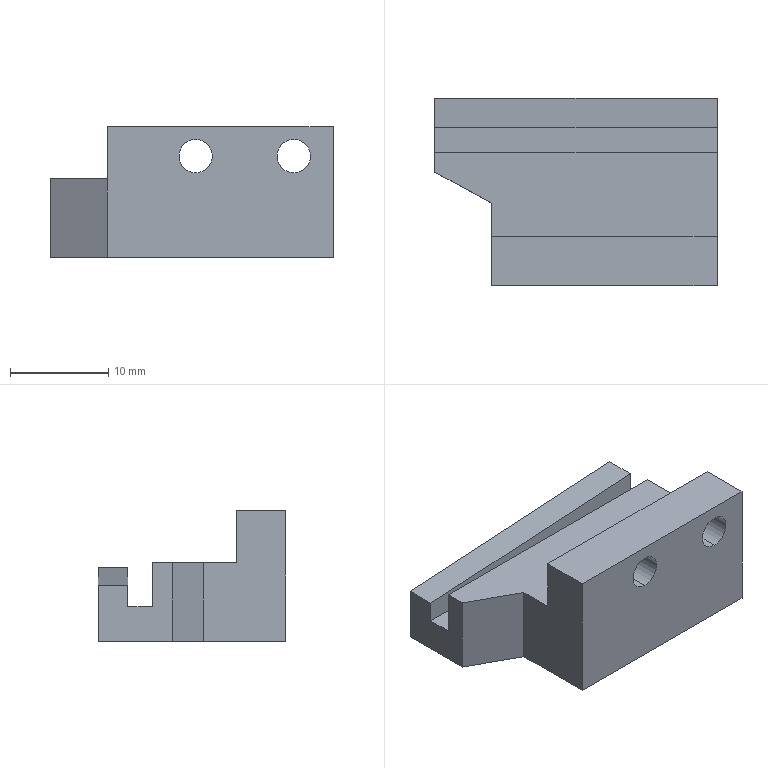Part | SolidWorks | features ICE 2, BaseBody 1 | 1 solid | 18 faces | box 28.739 x 19.08 x 13.3 mm | volume 4003 mm3 | plane 14 | cylinder 4 | commonest cylinder face diameters 3.4 x4
STEP:
#1=CARTESIAN_POINT('',(29.,5.,-1.));
#2=VERTEX_POINT('',#1);
#3=CARTESIAN_POINT('',(29.,5.,-4.4));
#4=VERTEX_POINT('',#3);
#5=CARTESIAN_POINT('',(29.,5.,-2.7));
#6=DIRECTION('',(0.,-1.,0.));
#7=DIRECTION('',(0.,0.,-1.));
#8=AXIS2_PLACEMENT_3D('',#5,#6,#7);
#9=CIRCLE('',#8,1.7);
#10=EDGE_CURVE('',#2,#4,#9,.T.);
#11=ORIENTED_EDGE('',*,*,#10,.F.);
#12=CARTESIAN_POINT('',(29.,0.,-1.));
#13=VERTEX_POINT('',#12);
#14=CARTESIAN_POINT('',(29.,0.,-1.));
#15=DIRECTION('',(0.,-1.,0.));
#16=VECTOR('',#15,1000.);
#17=LINE('',#14,#16);
#18=EDGE_CURVE('',#2,#13,#17,.T.);
#19=ORIENTED_EDGE('',*,*,#18,.T.);
#20=CARTESIAN_POINT('',(29.,0.,-4.4));
#21=VERTEX_POINT('',#20);
#22=CARTESIAN_POINT('',(29.,0.,-2.7));
#23=DIRECTION('',(0.,-1.,0.));
#24=DIRECTION('',(0.,0.,-1.));
#25=AXIS2_PLACEMENT_3D('',#22,#23,#24);
#26=CIRCLE('',#25,1.7);
#27=EDGE_CURVE('',#13,#21,#26,.T.);
#28=ORIENTED_EDGE('',*,*,#27,.T.);
#29=CARTESIAN_POINT('',(29.,0.,-4.4));
#30=DIRECTION('',(0.,-1.,0.));
#31=VECTOR('',#30,1000.);
#32=LINE('',#29,#31);
#33=EDGE_CURVE('',#4,#21,#32,.T.);
#34=ORIENTED_EDGE('',*,*,#33,.F.);
#35=EDGE_LOOP('',(#11,#19,#28,#34));
#36=FACE_OUTER_BOUND('',#35,.T.);
#37=CARTESIAN_POINT('',(29.,0.,-2.7));
#38=DIRECTION('',(0.,-1.,0.));
#39=DIRECTION('',(0.,0.,-1.));
#40=AXIS2_PLACEMENT_3D('',#37,#38,#39);
#41=CYLINDRICAL_SURFACE('',#40,1.7);
#42=ADVANCED_FACE('',(#36),#41,.F.);
#43=CARTESIAN_POINT('',(19.,5.,-1.));
#44=VERTEX_POINT('',#43);
#45=CARTESIAN_POINT('',(19.,5.,-4.4));
#46=VERTEX_POINT('',#45);
#47=CARTESIAN_POINT('',(19.,5.,-2.7));
#48=DIRECTION('',(0.,-1.,0.));
#49=DIRECTION('',(0.,0.,-1.));
#50=AXIS2_PLACEMENT_3D('',#47,#48,#49);
#51=CIRCLE('',#50,1.7);
#52=EDGE_CURVE('',#44,#46,#51,.T.);
#53=ORIENTED_EDGE('',*,*,#52,.F.);
#54=CARTESIAN_POINT('',(19.,0.,-1.));
#55=VERTEX_POINT('',#54);
#56=CARTESIAN_POINT('',(19.,0.,-1.));
#57=DIRECTION('',(0.,-1.,0.));
#58=VECTOR('',#57,1000.);
#59=LINE('',#56,#58);
#60=EDGE_CURVE('',#44,#55,#59,.T.);
#61=ORIENTED_EDGE('',*,*,#60,.T.);
#62=CARTESIAN_POINT('',(19.,0.,-4.4));
#63=VERTEX_POINT('',#62);
#64=CARTESIAN_POINT('',(19.,0.,-2.7));
#65=DIRECTION('',(0.,-1.,0.));
#66=DIRECTION('',(0.,0.,-1.));
#67=AXIS2_PLACEMENT_3D('',#64,#65,#66);
#68=CIRCLE('',#67,1.7);
#69=EDGE_CURVE('',#55,#63,#68,.T.);
#70=ORIENTED_EDGE('',*,*,#69,.T.);
#71=CARTESIAN_POINT('',(19.,0.,-4.4));
#72=DIRECTION('',(0.,-1.,0.));
#73=VECTOR('',#72,1000.);
#74=LINE('',#71,#73);
#75=EDGE_CURVE('',#46,#63,#74,.T.);
#76=ORIENTED_EDGE('',*,*,#75,.F.);
#77=EDGE_LOOP('',(#53,#61,#70,#76));
#78=FACE_OUTER_BOUND('',#77,.T.);
#79=CARTESIAN_POINT('',(19.,0.,-2.7));
#80=DIRECTION('',(0.,-1.,0.));
#81=DIRECTION('',(0.,0.,-1.));
#82=AXIS2_PLACEMENT_3D('',#79,#80,#81);
#83=CYLINDRICAL_SURFACE('',#82,1.7);
#84=ADVANCED_FACE('',(#78),#83,.F.);
#85=CARTESIAN_POINT('',(33.,19.08,-13.));
#86=VERTEX_POINT('',#85);
#87=CARTESIAN_POINT('',(33.,0.,-13.));
#88=VERTEX_POINT('',#87);
#89=CARTESIAN_POINT('',(33.,20.,-13.));
#90=DIRECTION('',(0.,-1.,0.));
#91=VECTOR('',#90,1000.);
#92=LINE('',#89,#91);
#93=EDGE_CURVE('',#86,#88,#92,.T.);
#94=ORIENTED_EDGE('',*,*,#93,.F.);
#95=CARTESIAN_POINT('',(33.,19.08,-5.5));
#96=VERTEX_POINT('',#95);
#97=CARTESIAN_POINT('',(33.,19.08,-6.5));
#98=DIRECTION('',(0.,0.,-1.));
#99=VECTOR('',#98,1000.);
#100=LINE('',#97,#99);
#101=EDGE_CURVE('',#96,#86,#100,.T.);
#102=ORIENTED_EDGE('',*,*,#101,.F.);
#103=CARTESIAN_POINT('',(33.,16.08,-5.5));
#104=VERTEX_POINT('',#103);
#105=CARTESIAN_POINT('',(33.,0.04878,-5.5));
#106=DIRECTION('',(0.,1.,0.));
#107=VECTOR('',#106,1000.);
#108=LINE('',#105,#107);
#109=EDGE_CURVE('',#104,#96,#108,.T.);
#110=ORIENTED_EDGE('',*,*,#109,.F.);
#111=CARTESIAN_POINT('',(33.,16.08,-9.5));
#112=VERTEX_POINT('',#111);
#113=CARTESIAN_POINT('',(33.,16.08,-9.5));
#114=DIRECTION('',(0.,0.,1.));
#115=VECTOR('',#114,1000.);
#116=LINE('',#113,#115);
#117=EDGE_CURVE('',#112,#104,#116,.T.);
#118=ORIENTED_EDGE('',*,*,#117,.F.);
#119=CARTESIAN_POINT('',(33.,13.58,-9.5));
#120=VERTEX_POINT('',#119);
#121=CARTESIAN_POINT('',(33.,16.08,-9.5));
#122=DIRECTION('',(0.,1.,0.));
#123=VECTOR('',#122,1000.);
#124=LINE('',#121,#123);
#125=EDGE_CURVE('',#120,#112,#124,.T.);
#126=ORIENTED_EDGE('',*,*,#125,.F.);
#127=CARTESIAN_POINT('',(33.,13.58,-5.));
#128=VERTEX_POINT('',#127);
#129=CARTESIAN_POINT('',(33.,13.58,-9.5));
#130=DIRECTION('',(0.,0.,1.));
#131=VECTOR('',#130,1000.);
#132=LINE('',#129,#131);
#133=EDGE_CURVE('',#120,#128,#132,.T.);
#134=ORIENTED_EDGE('',*,*,#133,.T.);
#135=CARTESIAN_POINT('',(33.,5.,-5.));
#136=VERTEX_POINT('',#135);
#137=CARTESIAN_POINT('',(33.,20.,-5.));
#138=DIRECTION('',(0.,1.,0.));
#139=VECTOR('',#138,1000.);
#140=LINE('',#137,#139);
#141=EDGE_CURVE('',#136,#128,#140,.T.);
#142=ORIENTED_EDGE('',*,*,#141,.F.);
#143=CARTESIAN_POINT('',(33.,5.,0.3));
#144=VERTEX_POINT('',#143);
#145=CARTESIAN_POINT('',(33.,5.,-5.));
#146=DIRECTION('',(0.,0.,1.));
#147=VECTOR('',#146,1000.);
#148=LINE('',#145,#147);
#149=EDGE_CURVE('',#136,#144,#148,.T.);
#150=ORIENTED_EDGE('',*,*,#149,.T.);
#151=CARTESIAN_POINT('',(33.,0.,0.3));
#152=VERTEX_POINT('',#151);
#153=CARTESIAN_POINT('',(33.,5.,0.3));
#154=DIRECTION('',(0.,1.,0.));
#155=VECTOR('',#154,1000.);
#156=LINE('',#153,#155);
#157=EDGE_CURVE('',#152,#144,#156,.T.);
#158=ORIENTED_EDGE('',*,*,#157,.F.);
#159=CARTESIAN_POINT('',(33.,0.,0.));
#160=DIRECTION('',(0.,0.,-1.));
#161=VECTOR('',#160,1000.);
#162=LINE('',#159,#161);
#163=EDGE_CURVE('',#152,#88,#162,.T.);
#164=ORIENTED_EDGE('',*,*,#163,.T.);
#165=EDGE_LOOP('',(#94,#102,#110,#118,#126,#134,#142,#150,#158,#164));
#166=FACE_OUTER_BOUND('',#165,.T.);
#167=CARTESIAN_POINT('',(33.,20.,0.));
#168=DIRECTION('',(-1.,0.,0.));
#169=DIRECTION('',(0.,0.,1.));
#170=AXIS2_PLACEMENT_3D('',#167,#168,#169);
#171=PLANE('',#170);
#172=ADVANCED_FACE('',(#166),#171,.F.);
#173=CARTESIAN_POINT('',(4.261,11.561,-13.));
#174=VERTEX_POINT('',#173);
#175=CARTESIAN_POINT('',(10.,8.409,-13.));
#176=VERTEX_POINT('',#175);
#177=CARTESIAN_POINT('',(-2.244,15.136,-13.));
#178=DIRECTION('',(0.8764,-0.4815,0.));
#179=VECTOR('',#178,1000.);
#180=LINE('',#177,#179);
#181=EDGE_CURVE('',#174,#176,#180,.T.);
#182=ORIENTED_EDGE('',*,*,#181,.F.);
#183=CARTESIAN_POINT('',(4.261,19.08,-13.));
#184=VERTEX_POINT('',#183);
#185=CARTESIAN_POINT('',(4.261,19.08,-13.));
#186=DIRECTION('',(0.,-1.,0.));
#187=VECTOR('',#186,1000.);
#188=LINE('',#185,#187);
#189=EDGE_CURVE('',#184,#174,#188,.T.);
#190=ORIENTED_EDGE('',*,*,#189,.F.);
#191=CARTESIAN_POINT('',(0.,19.08,-13.));
#192=DIRECTION('',(1.,0.,0.));
#193=VECTOR('',#192,1000.);
#194=LINE('',#191,#193);
#195=EDGE_CURVE('',#184,#86,#194,.T.);
#196=ORIENTED_EDGE('',*,*,#195,.T.);
#197=ORIENTED_EDGE('',*,*,#93,.T.);
#198=CARTESIAN_POINT('',(10.,0.,-13.));
#199=VERTEX_POINT('',#198);
#200=CARTESIAN_POINT('',(33.,0.,-13.));
#201=DIRECTION('',(-1.,0.,0.));
#202=VECTOR('',#201,1000.);
#203=LINE('',#200,#202);
#204=EDGE_CURVE('',#88,#199,#203,.T.);
#205=ORIENTED_EDGE('',*,*,#204,.T.);
#206=CARTESIAN_POINT('',(10.,0.,-13.));
#207=DIRECTION('',(0.,-1.,0.));
#208=VECTOR('',#207,1000.);
#209=LINE('',#206,#208);
#210=EDGE_CURVE('',#176,#199,#209,.T.);
#211=ORIENTED_EDGE('',*,*,#210,.F.);
#212=EDGE_LOOP('',(#182,#190,#196,#197,#205,#211));
#213=FACE_OUTER_BOUND('',#212,.T.);
#214=CARTESIAN_POINT('',(33.,20.,-13.));
#215=DIRECTION('',(0.,0.,1.));
#216=DIRECTION('',(1.,0.,0.));
#217=AXIS2_PLACEMENT_3D('',#214,#215,#216);
#218=PLANE('',#217);
#219=ADVANCED_FACE('',(#213),#218,.F.);
#220=CARTESIAN_POINT('',(29.,0.,-2.7));
#221=DIRECTION('',(0.,-1.,0.));
#222=DIRECTION('',(0.,0.,-1.));
#223=AXIS2_PLACEMENT_3D('',#220,#221,#222);
#224=CIRCLE('',#223,1.7);
#225=EDGE_CURVE('',#21,#13,#224,.T.);
#226=ORIENTED_EDGE('',*,*,#225,.F.);
#227=ORIENTED_EDGE('',*,*,#27,.F.);
#228=EDGE_LOOP('',(#226,#227));
#229=FACE_BOUND('',#228,.T.);
#230=CARTESIAN_POINT('',(19.,0.,-2.7));
#231=DIRECTION('',(0.,-1.,0.));
#232=DIRECTION('',(0.,0.,-1.));
#233=AXIS2_PLACEMENT_3D('',#230,#231,#232);
#234=CIRCLE('',#233,1.7);
#235=EDGE_CURVE('',#63,#55,#234,.T.);
#236=ORIENTED_EDGE('',*,*,#235,.F.);
#237=ORIENTED_EDGE('',*,*,#69,.F.);
#238=EDGE_LOOP('',(#236,#237));
#239=FACE_BOUND('',#238,.T.);
#240=ORIENTED_EDGE('',*,*,#163,.F.);
#241=CARTESIAN_POINT('',(10.,0.,0.3));
#242=VERTEX_POINT('',#241);
#243=CARTESIAN_POINT('',(33.,0.,0.3));
#244=DIRECTION('',(1.,0.,0.));
#245=VECTOR('',#244,1000.);
#246=LINE('',#243,#245);
#247=EDGE_CURVE('',#242,#152,#246,.T.);
#248=ORIENTED_EDGE('',*,*,#247,.F.);
#249=CARTESIAN_POINT('',(10.,0.,-1.7));
#250=DIRECTION('',(0.,0.,-1.));
#251=VECTOR('',#250,1000.);
#252=LINE('',#249,#251);
#253=EDGE_CURVE('',#242,#199,#252,.T.);
#254=ORIENTED_EDGE('',*,*,#253,.T.);
#255=ORIENTED_EDGE('',*,*,#204,.F.);
#256=EDGE_LOOP('',(#240,#248,#254,#255));
#257=FACE_OUTER_BOUND('',#256,.T.);
#258=CARTESIAN_POINT('',(0.,0.,0.));
#259=DIRECTION('',(0.,1.,0.));
#260=DIRECTION('',(0.,0.,1.));
#261=AXIS2_PLACEMENT_3D('',#258,#259,#260);
#262=PLANE('',#261);
#263=ADVANCED_FACE('',(#229,#239,#257),#262,.F.);
#264=CARTESIAN_POINT('',(29.,5.,-2.7));
#265=DIRECTION('',(0.,-1.,0.));
#266=DIRECTION('',(0.,0.,-1.));
#267=AXIS2_PLACEMENT_3D('',#264,#265,#266);
#268=CIRCLE('',#267,1.7);
#269=EDGE_CURVE('',#4,#2,#268,.T.);
#270=ORIENTED_EDGE('',*,*,#269,.T.);
#271=ORIENTED_EDGE('',*,*,#10,.T.);
#272=EDGE_LOOP('',(#270,#271));
#273=FACE_BOUND('',#272,.T.);
#274=CARTESIAN_POINT('',(19.,5.,-2.7));
#275=DIRECTION('',(0.,-1.,0.));
#276=DIRECTION('',(0.,0.,-1.));
#277=AXIS2_PLACEMENT_3D('',#274,#275,#276);
#278=CIRCLE('',#277,1.7);
#279=EDGE_CURVE('',#46,#44,#278,.T.);
#280=ORIENTED_EDGE('',*,*,#279,.T.);
#281=ORIENTED_EDGE('',*,*,#52,.T.);
#282=EDGE_LOOP('',(#280,#281));
#283=FACE_BOUND('',#282,.T.);
#284=CARTESIAN_POINT('',(10.,5.,-5.));
#285=VERTEX_POINT('',#284);
#286=CARTESIAN_POINT('',(0.,5.,-5.));
#287=DIRECTION('',(1.,0.,0.));
#288=VECTOR('',#287,1000.);
#289=LINE('',#286,#288);
#290=EDGE_CURVE('',#285,#136,#289,.T.);
#291=ORIENTED_EDGE('',*,*,#290,.F.);
#292=CARTESIAN_POINT('',(10.,5.,0.3));
#293=VERTEX_POINT('',#292);
#294=CARTESIAN_POINT('',(10.,5.,-5.));
#295=DIRECTION('',(0.,0.,1.));
#296=VECTOR('',#295,1000.);
#297=LINE('',#294,#296);
#298=EDGE_CURVE('',#285,#293,#297,.T.);
#299=ORIENTED_EDGE('',*,*,#298,.T.);
#300=CARTESIAN_POINT('',(33.,5.,0.3));
#301=DIRECTION('',(-1.,0.,0.));
#302=VECTOR('',#301,1000.);
#303=LINE('',#300,#302);
#304=EDGE_CURVE('',#144,#293,#303,.T.);
#305=ORIENTED_EDGE('',*,*,#304,.F.);
#306=ORIENTED_EDGE('',*,*,#149,.F.);
#307=EDGE_LOOP('',(#291,#299,#305,#306));
#308=FACE_OUTER_BOUND('',#307,.T.);
#309=CARTESIAN_POINT('',(0.,5.,-5.));
#310=DIRECTION('',(0.,-1.,0.));
#311=DIRECTION('',(0.,0.,-1.));
#312=AXIS2_PLACEMENT_3D('',#309,#310,#311);
#313=PLANE('',#312);
#314=ADVANCED_FACE('',(#273,#283,#308),#313,.F.);
#315=CARTESIAN_POINT('',(4.261,11.561,-5.));
#316=VERTEX_POINT('',#315);
#317=CARTESIAN_POINT('',(4.261,13.58,-5.));
#318=VERTEX_POINT('',#317);
#319=CARTESIAN_POINT('',(4.261,5.,-5.));
#320=DIRECTION('',(0.,1.,0.));
#321=VECTOR('',#320,1000.);
#322=LINE('',#319,#321);
#323=EDGE_CURVE('',#316,#318,#322,.T.);
#324=ORIENTED_EDGE('',*,*,#323,.F.);
#325=CARTESIAN_POINT('',(10.,8.409,-5.));
#326=VERTEX_POINT('',#325);
#327=CARTESIAN_POINT('',(3.757,11.839,-5.));
#328=DIRECTION('',(-0.8764,0.4815,0.));
#329=VECTOR('',#328,1000.);
#330=LINE('',#327,#329);
#331=EDGE_CURVE('',#326,#316,#330,.T.);
#332=ORIENTED_EDGE('',*,*,#331,.F.);
#333=CARTESIAN_POINT('',(10.,5.,-5.));
#334=DIRECTION('',(0.,1.,0.));
#335=VECTOR('',#334,1000.);
#336=LINE('',#333,#335);
#337=EDGE_CURVE('',#285,#326,#336,.T.);
#338=ORIENTED_EDGE('',*,*,#337,.F.);
#339=ORIENTED_EDGE('',*,*,#290,.T.);
#340=ORIENTED_EDGE('',*,*,#141,.T.);
#341=CARTESIAN_POINT('',(0.,13.58,-5.));
#342=DIRECTION('',(1.,0.,0.));
#343=VECTOR('',#342,1000.);
#344=LINE('',#341,#343);
#345=EDGE_CURVE('',#318,#128,#344,.T.);
#346=ORIENTED_EDGE('',*,*,#345,.F.);
#347=EDGE_LOOP('',(#324,#332,#338,#339,#340,#346));
#348=FACE_OUTER_BOUND('',#347,.T.);
#349=CARTESIAN_POINT('',(0.,5.,-5.));
#350=DIRECTION('',(0.,0.,1.));
#351=DIRECTION('',(1.,0.,0.));
#352=AXIS2_PLACEMENT_3D('',#349,#350,#351);
#353=PLANE('',#352);
#354=ADVANCED_FACE('',(#348),#353,.T.);
#355=CARTESIAN_POINT('',(4.261,16.08,-7.296));
#356=VERTEX_POINT('',#355);
#357=CARTESIAN_POINT('',(33.,16.08,-5.5));
#358=DIRECTION('',(-0.9981,0.,-0.06238));
#359=VECTOR('',#358,1000.);
#360=LINE('',#357,#359);
#361=EDGE_CURVE('',#104,#356,#360,.T.);
#362=ORIENTED_EDGE('',*,*,#361,.T.);
#363=CARTESIAN_POINT('',(4.261,16.08,-9.5));
#364=VERTEX_POINT('',#363);
#365=CARTESIAN_POINT('',(4.261,16.08,-9.5));
#366=DIRECTION('',(0.,0.,-1.));
#367=VECTOR('',#366,1000.);
#368=LINE('',#365,#367);
#369=EDGE_CURVE('',#356,#364,#368,.T.);
#370=ORIENTED_EDGE('',*,*,#369,.T.);
#371=CARTESIAN_POINT('',(0.,16.08,-9.5));
#372=DIRECTION('',(-1.,0.,0.));
#373=VECTOR('',#372,1000.);
#374=LINE('',#371,#373);
#375=EDGE_CURVE('',#112,#364,#374,.T.);
#376=ORIENTED_EDGE('',*,*,#375,.F.);
#377=ORIENTED_EDGE('',*,*,#117,.T.);
#378=EDGE_LOOP('',(#362,#370,#376,#377));
#379=FACE_OUTER_BOUND('',#378,.T.);
#380=CARTESIAN_POINT('',(0.,16.08,-9.5));
#381=DIRECTION('',(0.,1.,0.));
#382=DIRECTION('',(0.,0.,1.));
#383=AXIS2_PLACEMENT_3D('',#380,#381,#382);
#384=PLANE('',#383);
#385=ADVANCED_FACE('',(#379),#384,.F.);
#386=CARTESIAN_POINT('',(4.261,13.58,-9.5));
#387=VERTEX_POINT('',#386);
#388=CARTESIAN_POINT('',(0.,13.58,-9.5));
#389=DIRECTION('',(1.,0.,0.));
#390=VECTOR('',#389,1000.);
#391=LINE('',#388,#390);
#392=EDGE_CURVE('',#387,#120,#391,.T.);
#393=ORIENTED_EDGE('',*,*,#392,.F.);
#394=CARTESIAN_POINT('',(4.261,13.58,-9.5));
#395=DIRECTION('',(0.,0.,1.));
#396=VECTOR('',#395,1000.);
#397=LINE('',#394,#396);
#398=EDGE_CURVE('',#387,#318,#397,.T.);
#399=ORIENTED_EDGE('',*,*,#398,.T.);
#400=ORIENTED_EDGE('',*,*,#345,.T.);
#401=ORIENTED_EDGE('',*,*,#133,.F.);
#402=EDGE_LOOP('',(#393,#399,#400,#401));
#403=FACE_OUTER_BOUND('',#402,.T.);
#404=CARTESIAN_POINT('',(0.,13.58,-9.5));
#405=DIRECTION('',(0.,-1.,0.));
#406=DIRECTION('',(0.,0.,-1.));
#407=AXIS2_PLACEMENT_3D('',#404,#405,#406);
#408=PLANE('',#407);
#409=ADVANCED_FACE('',(#403),#408,.F.);
#410=CARTESIAN_POINT('',(4.261,13.58,-9.5));
#411=DIRECTION('',(0.,1.,0.));
#412=VECTOR('',#411,1000.);
#413=LINE('',#410,#412);
#414=EDGE_CURVE('',#387,#364,#413,.T.);
#415=ORIENTED_EDGE('',*,*,#414,.F.);
#416=ORIENTED_EDGE('',*,*,#392,.T.);
#417=ORIENTED_EDGE('',*,*,#125,.T.);
#418=ORIENTED_EDGE('',*,*,#375,.T.);
#419=EDGE_LOOP('',(#415,#416,#417,#418));
#420=FACE_OUTER_BOUND('',#419,.T.);
#421=CARTESIAN_POINT('',(0.,13.58,-9.5));
#422=DIRECTION('',(0.,0.,1.));
#423=DIRECTION('',(1.,0.,0.));
#424=AXIS2_PLACEMENT_3D('',#421,#422,#423);
#425=PLANE('',#424);
#426=ADVANCED_FACE('',(#420),#425,.T.);
#427=CARTESIAN_POINT('',(10.,5.,0.3));
#428=DIRECTION('',(0.,1.,0.));
#429=VECTOR('',#428,1000.);
#430=LINE('',#427,#429);
#431=EDGE_CURVE('',#242,#293,#430,.T.);
#432=ORIENTED_EDGE('',*,*,#431,.F.);
#433=ORIENTED_EDGE('',*,*,#247,.T.);
#434=ORIENTED_EDGE('',*,*,#157,.T.);
#435=ORIENTED_EDGE('',*,*,#304,.T.);
#436=EDGE_LOOP('',(#432,#433,#434,#435));
#437=FACE_OUTER_BOUND('',#436,.T.);
#438=CARTESIAN_POINT('',(33.,5.,0.3));
#439=DIRECTION('',(0.,0.,1.));
#440=DIRECTION('',(1.,0.,0.));
#441=AXIS2_PLACEMENT_3D('',#438,#439,#440);
#442=PLANE('',#441);
#443=ADVANCED_FACE('',(#437),#442,.T.);
#444=CARTESIAN_POINT('',(4.261,19.08,-7.296));
#445=VERTEX_POINT('',#444);
#446=CARTESIAN_POINT('',(4.261,19.08,-3.));
#447=DIRECTION('',(0.,0.,-1.));
#448=VECTOR('',#447,1000.);
#449=LINE('',#446,#448);
#450=EDGE_CURVE('',#445,#184,#449,.T.);
#451=ORIENTED_EDGE('',*,*,#450,.F.);
#452=CARTESIAN_POINT('',(33.,19.08,-5.5));
#453=DIRECTION('',(0.9981,0.,0.06238));
#454=VECTOR('',#453,1000.);
#455=LINE('',#452,#454);
#456=EDGE_CURVE('',#445,#96,#455,.T.);
#457=ORIENTED_EDGE('',*,*,#456,.T.);
#458=ORIENTED_EDGE('',*,*,#101,.T.);
#459=ORIENTED_EDGE('',*,*,#195,.F.);
#460=EDGE_LOOP('',(#451,#457,#458,#459));
#461=FACE_OUTER_BOUND('',#460,.T.);
#462=CARTESIAN_POINT('',(0.,19.08,-6.5));
#463=DIRECTION('',(0.,-1.,0.));
#464=DIRECTION('',(0.,0.,-1.));
#465=AXIS2_PLACEMENT_3D('',#462,#463,#464);
#466=PLANE('',#465);
#467=ADVANCED_FACE('',(#461),#466,.F.);
#468=ORIENTED_EDGE('',*,*,#60,.F.);
#469=ORIENTED_EDGE('',*,*,#279,.F.);
#470=ORIENTED_EDGE('',*,*,#75,.T.);
#471=ORIENTED_EDGE('',*,*,#235,.T.);
#472=EDGE_LOOP('',(#468,#469,#470,#471));
#473=FACE_OUTER_BOUND('',#472,.T.);
#474=CARTESIAN_POINT('',(19.,0.,-2.7));
#475=DIRECTION('',(0.,-1.,0.));
#476=DIRECTION('',(0.,0.,-1.));
#477=AXIS2_PLACEMENT_3D('',#474,#475,#476);
#478=CYLINDRICAL_SURFACE('',#477,1.7);
#479=ADVANCED_FACE('',(#473),#478,.F.);
#480=ORIENTED_EDGE('',*,*,#18,.F.);
#481=ORIENTED_EDGE('',*,*,#269,.F.);
#482=ORIENTED_EDGE('',*,*,#33,.T.);
#483=ORIENTED_EDGE('',*,*,#225,.T.);
#484=EDGE_LOOP('',(#480,#481,#482,#483));
#485=FACE_OUTER_BOUND('',#484,.T.);
#486=CARTESIAN_POINT('',(29.,0.,-2.7));
#487=DIRECTION('',(0.,-1.,0.));
#488=DIRECTION('',(0.,0.,-1.));
#489=AXIS2_PLACEMENT_3D('',#486,#487,#488);
#490=CYLINDRICAL_SURFACE('',#489,1.7);
#491=ADVANCED_FACE('',(#485),#490,.F.);
#492=ORIENTED_EDGE('',*,*,#331,.T.);
#493=CARTESIAN_POINT('',(4.261,11.561,0.3));
#494=DIRECTION('',(0.,0.,-1.));
#495=VECTOR('',#494,1000.);
#496=LINE('',#493,#495);
#497=EDGE_CURVE('',#316,#174,#496,.T.);
#498=ORIENTED_EDGE('',*,*,#497,.T.);
#499=ORIENTED_EDGE('',*,*,#181,.T.);
#500=CARTESIAN_POINT('',(10.,8.409,0.3));
#501=DIRECTION('',(0.,0.,-1.));
#502=VECTOR('',#501,1000.);
#503=LINE('',#500,#502);
#504=EDGE_CURVE('',#326,#176,#503,.T.);
#505=ORIENTED_EDGE('',*,*,#504,.F.);
#506=EDGE_LOOP('',(#492,#498,#499,#505));
#507=FACE_OUTER_BOUND('',#506,.T.);
#508=CARTESIAN_POINT('',(-2.244,15.136,0.3));
#509=DIRECTION('',(0.4815,0.8764,0.));
#510=DIRECTION('',(-0.8764,0.4815,0.));
#511=AXIS2_PLACEMENT_3D('',#508,#509,#510);
#512=PLANE('',#511);
#513=ADVANCED_FACE('',(#507),#512,.F.);
#514=ORIENTED_EDGE('',*,*,#337,.T.);
#515=ORIENTED_EDGE('',*,*,#504,.T.);
#516=ORIENTED_EDGE('',*,*,#210,.T.);
#517=ORIENTED_EDGE('',*,*,#253,.F.);
#518=ORIENTED_EDGE('',*,*,#431,.T.);
#519=ORIENTED_EDGE('',*,*,#298,.F.);
#520=EDGE_LOOP('',(#514,#515,#516,#517,#518,#519));
#521=FACE_OUTER_BOUND('',#520,.T.);
#522=CARTESIAN_POINT('',(10.,0.,0.3));
#523=DIRECTION('',(1.,0.,0.));
#524=DIRECTION('',(0.,0.,-1.));
#525=AXIS2_PLACEMENT_3D('',#522,#523,#524);
#526=PLANE('',#525);
#527=ADVANCED_FACE('',(#521),#526,.F.);
#528=ORIENTED_EDGE('',*,*,#369,.F.);
#529=CARTESIAN_POINT('',(4.261,3.317,-7.296));
#530=DIRECTION('',(0.,1.,0.));
#531=VECTOR('',#530,1000.);
#532=LINE('',#529,#531);
#533=EDGE_CURVE('',#356,#445,#532,.T.);
#534=ORIENTED_EDGE('',*,*,#533,.T.);
#535=ORIENTED_EDGE('',*,*,#450,.T.);
#536=ORIENTED_EDGE('',*,*,#189,.T.);
#537=ORIENTED_EDGE('',*,*,#497,.F.);
#538=ORIENTED_EDGE('',*,*,#323,.T.);
#539=ORIENTED_EDGE('',*,*,#398,.F.);
#540=ORIENTED_EDGE('',*,*,#414,.T.);
#541=EDGE_LOOP('',(#528,#534,#535,#536,#537,#538,#539,#540));
#542=FACE_OUTER_BOUND('',#541,.T.);
#543=CARTESIAN_POINT('',(4.261,19.08,-3.));
#544=DIRECTION('',(1.,0.,0.));
#545=DIRECTION('',(0.,1.,0.));
#546=AXIS2_PLACEMENT_3D('',#543,#544,#545);
#547=PLANE('',#546);
#548=ADVANCED_FACE('',(#542),#547,.F.);
#549=ORIENTED_EDGE('',*,*,#361,.F.);
#550=ORIENTED_EDGE('',*,*,#109,.T.);
#551=ORIENTED_EDGE('',*,*,#456,.F.);
#552=ORIENTED_EDGE('',*,*,#533,.F.);
#553=EDGE_LOOP('',(#549,#550,#551,#552));
#554=FACE_OUTER_BOUND('',#553,.T.);
#555=CARTESIAN_POINT('',(33.,0.04878,-5.5));
#556=DIRECTION('',(-0.06238,0.,0.9981));
#557=DIRECTION('',(0.9981,0.,0.06238));
#558=AXIS2_PLACEMENT_3D('',#555,#556,#557);
#559=PLANE('',#558);
#560=ADVANCED_FACE('',(#554),#559,.T.);
#561=CLOSED_SHELL('',(#42,#84,#172,#219,#263,#314,#354,#385,#409,#426,#443,#467,#479,#491,#513,#527,#548,#560));
#562=MANIFOLD_SOLID_BREP('',#561);
#563=CARTESIAN_POINT('',(0.,0.,0.));
#564=DIRECTION('',(0.,0.,1.));
#565=DIRECTION('',(1.,0.,0.));
#566=AXIS2_PLACEMENT_3D('',#563,#564,#565);
#567=(LENGTH_UNIT()NAMED_UNIT(*)SI_UNIT(.MILLI.,.METRE.));
#568=UNCERTAINTY_MEASURE_WITH_UNIT(LENGTH_MEASURE(0.00001),#567,'','');
#569=(NAMED_UNIT(*)PLANE_ANGLE_UNIT()SI_UNIT($,.RADIAN.));
#570=(NAMED_UNIT(*)SI_UNIT($,.STERADIAN.)SOLID_ANGLE_UNIT());
#571=(GEOMETRIC_REPRESENTATION_CONTEXT(3)GLOBAL_UNCERTAINTY_ASSIGNED_CONTEXT((#568))GLOBAL_UNIT_ASSIGNED_CONTEXT((#567,#569,#570))REPRESENTATION_CONTEXT('',''));
#572=ADVANCED_BREP_SHAPE_REPRESENTATION('',(#562,#566),#571);